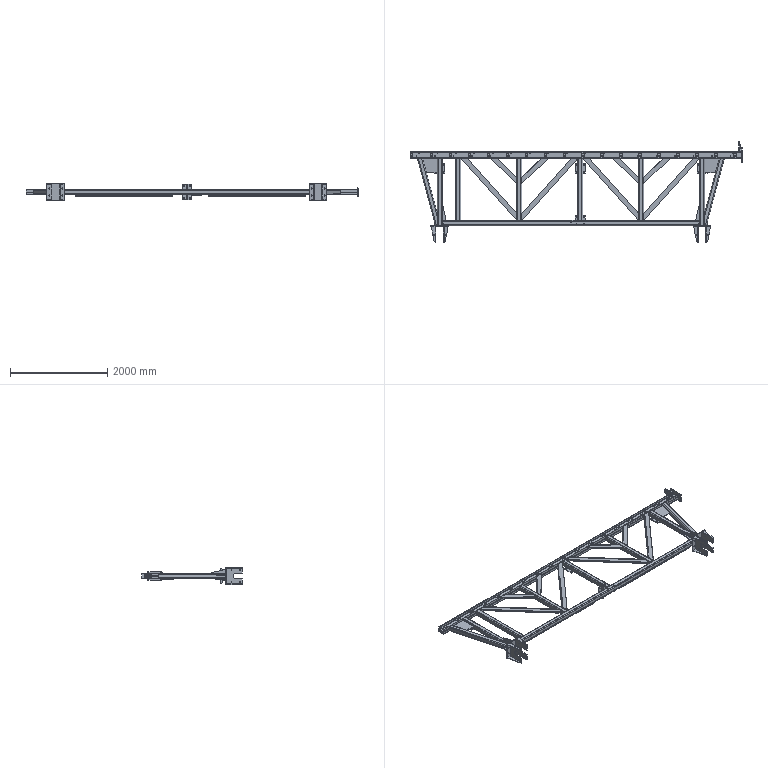Part | SolidWorks | features ReferencePattern 15, LocalLPattern 6, MateUpdatePoint 2 | 93 solids | 1194 faces | box 6830 x 2073 x 360 mm | volume 92757683 mm3 | plane 642 | cylinder 552 | commonest cylinder face diameters 16 x146 13 x144 21 x64 17 x38 26.12 x36 38.12 x36